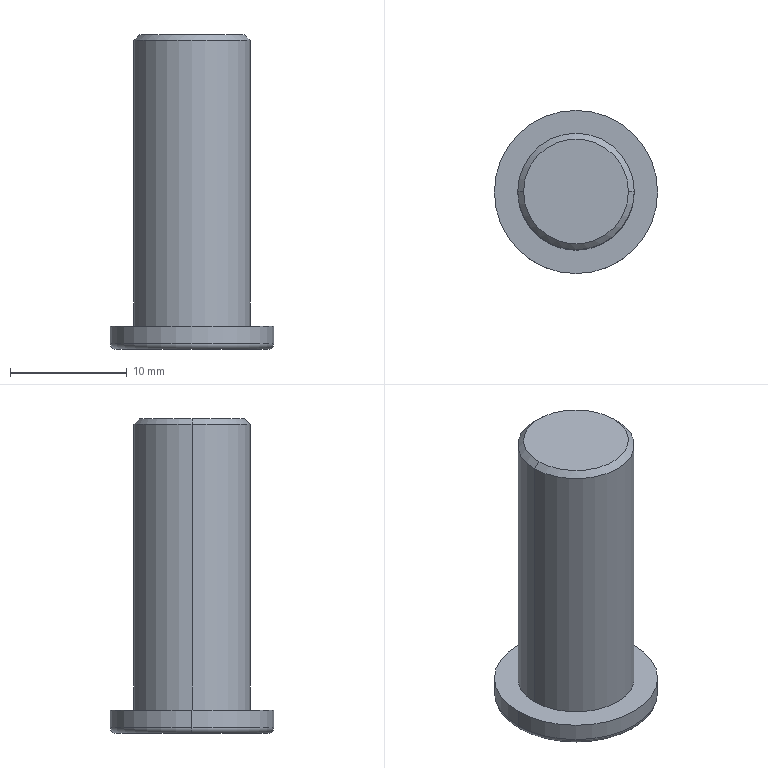Part | STEP file | BCC3 H11_4 | 1 solid | 11 faces | box 14 x 14 x 27 mm | volume 2265 mm3 | cylinder 4 | plane 3 | torus 2 | cone 2 | commonest cylinder face diameters 10 x2 14 x2
STEP:
#1=CARTESIAN_POINT('',(0.,0.,0.));
#2=DIRECTION('',(0.,0.,1.));
#3=DIRECTION('',(1.,0.,0.));
#4=AXIS2_PLACEMENT_3D('',#1,#2,#3);
#5=CARTESIAN_POINT('',(-6.5,0.,-2.));
#6=VERTEX_POINT('',#5);
#7=CARTESIAN_POINT('',(6.5,0.,-2.));
#8=VERTEX_POINT('',#7);
#9=CARTESIAN_POINT('',(0.,0.,-2.));
#10=DIRECTION('',(0.,0.,-1.));
#11=DIRECTION('',(1.,0.,0.));
#12=AXIS2_PLACEMENT_3D('',#9,#10,#11);
#13=CIRCLE('',#12,6.5);
#14=CARTESIAN_POINT('',(0.,0.,-1.5));
#15=DIRECTION('',(0.,0.,1.));
#16=DIRECTION('',(1.,0.,0.));
#17=AXIS2_PLACEMENT_3D('',#14,#15,#16);
#18=TOROIDAL_SURFACE('',#17,6.5,0.5);
#19=CARTESIAN_POINT('',(6.283,4.712));
#20=DIRECTION('',(-1.,0.));
#21=VECTOR('',#20,1.);
#22=LINE('',#19,#21);
#23=(GEOMETRIC_REPRESENTATION_CONTEXT(2)PARAMETRIC_REPRESENTATION_CONTEXT()REPRESENTATION_CONTEXT('',''));
#24=DEFINITIONAL_REPRESENTATION('',(#22),#23);
#25=PCURVE('',#18,#24);
#26=CARTESIAN_POINT('',(0.,0.,-2.));
#27=DIRECTION('',(0.,0.,1.));
#28=DIRECTION('',(1.,0.,0.));
#29=AXIS2_PLACEMENT_3D('',#26,#27,#28);
#30=PLANE('',#29);
#31=CARTESIAN_POINT('',(6.5,0.));
#32=CARTESIAN_POINT('',(6.5,-11.258));
#33=CARTESIAN_POINT('',(-3.25,-5.629));
#34=CARTESIAN_POINT('',(-13.,0.));
#35=CARTESIAN_POINT('',(-3.25,5.629));
#36=CARTESIAN_POINT('',(6.5,11.258));
#37=CARTESIAN_POINT('',(6.5,0.));
#38=(BOUNDED_CURVE()B_SPLINE_CURVE(2,(#31,#32,#33,#34,#35,#36,#37),.UNSPECIFIED.,.T.,.F.)B_SPLINE_CURVE_WITH_KNOTS((1,2,2,2,2,1),(-2.094,0.,2.094,4.189,6.283,8.378),.UNSPECIFIED.)CURVE()GEOMETRIC_REPRESENTATION_ITEM()RATIONAL_B_SPLINE_CURVE((1.,0.5,1.,0.5,1.,0.5,1.))REPRESENTATION_ITEM(''));
#39=(GEOMETRIC_REPRESENTATION_CONTEXT(2)PARAMETRIC_REPRESENTATION_CONTEXT()REPRESENTATION_CONTEXT('',''));
#40=DEFINITIONAL_REPRESENTATION('',(#38),#39);
#41=PCURVE('',#30,#40);
#42=SURFACE_CURVE('',#13,(#25,#41),.PCURVE_S1.);
#43=EDGE_CURVE('',#6,#8,#42,.T.);
#44=ORIENTED_EDGE('',*,*,#43,.F.);
#45=CARTESIAN_POINT('',(-7.,0.,-1.5));
#46=VERTEX_POINT('',#45);
#47=CARTESIAN_POINT('',(-6.5,0.,-1.5));
#48=DIRECTION('',(0.,1.,0.));
#49=DIRECTION('',(-1.,0.,0.));
#50=AXIS2_PLACEMENT_3D('',#47,#48,#49);
#51=CIRCLE('',#50,0.5);
#52=CARTESIAN_POINT('',(3.142,0.));
#53=DIRECTION('',(0.,1.));
#54=VECTOR('',#53,1.);
#55=LINE('',#52,#54);
#56=(GEOMETRIC_REPRESENTATION_CONTEXT(2)PARAMETRIC_REPRESENTATION_CONTEXT()REPRESENTATION_CONTEXT('',''));
#57=DEFINITIONAL_REPRESENTATION('',(#55),#56);
#58=PCURVE('',#18,#57);
#59=CARTESIAN_POINT('',(0.,0.,-1.5));
#60=DIRECTION('',(0.,0.,1.));
#61=DIRECTION('',(1.,0.,0.));
#62=AXIS2_PLACEMENT_3D('',#59,#60,#61);
#63=TOROIDAL_SURFACE('',#62,6.5,0.5);
#64=CARTESIAN_POINT('',(3.142,0.));
#65=DIRECTION('',(0.,1.));
#66=VECTOR('',#65,1.);
#67=LINE('',#64,#66);
#68=(GEOMETRIC_REPRESENTATION_CONTEXT(2)PARAMETRIC_REPRESENTATION_CONTEXT()REPRESENTATION_CONTEXT('',''));
#69=DEFINITIONAL_REPRESENTATION('',(#67),#68);
#70=PCURVE('',#63,#69);
#71=SURFACE_CURVE('',#51,(#58,#70),.PCURVE_S1.);
#72=EDGE_CURVE('',#6,#46,#71,.T.);
#73=ORIENTED_EDGE('',*,*,#72,.T.);
#74=CARTESIAN_POINT('',(7.,0.,-1.5));
#75=VERTEX_POINT('',#74);
#76=CARTESIAN_POINT('',(0.,0.,-1.5));
#77=DIRECTION('',(0.,0.,1.));
#78=DIRECTION('',(1.,0.,0.));
#79=AXIS2_PLACEMENT_3D('',#76,#77,#78);
#80=CIRCLE('',#79,7.);
#81=CARTESIAN_POINT('',(0.,6.283));
#82=DIRECTION('',(1.,0.));
#83=VECTOR('',#82,1.);
#84=LINE('',#81,#83);
#85=(GEOMETRIC_REPRESENTATION_CONTEXT(2)PARAMETRIC_REPRESENTATION_CONTEXT()REPRESENTATION_CONTEXT('',''));
#86=DEFINITIONAL_REPRESENTATION('',(#84),#85);
#87=PCURVE('',#18,#86);
#88=CARTESIAN_POINT('',(0.,0.,-2.));
#89=DIRECTION('',(0.,0.,1.));
#90=DIRECTION('',(1.,0.,0.));
#91=AXIS2_PLACEMENT_3D('',#88,#89,#90);
#92=CYLINDRICAL_SURFACE('',#91,7.);
#93=CARTESIAN_POINT('',(0.,0.5));
#94=DIRECTION('',(1.,0.));
#95=VECTOR('',#94,1.);
#96=LINE('',#93,#95);
#97=(GEOMETRIC_REPRESENTATION_CONTEXT(2)PARAMETRIC_REPRESENTATION_CONTEXT()REPRESENTATION_CONTEXT('',''));
#98=DEFINITIONAL_REPRESENTATION('',(#96),#97);
#99=PCURVE('',#92,#98);
#100=SURFACE_CURVE('',#80,(#87,#99),.PCURVE_S1.);
#101=EDGE_CURVE('',#75,#46,#100,.T.);
#102=ORIENTED_EDGE('',*,*,#101,.F.);
#103=CARTESIAN_POINT('',(6.5,0.,-1.5));
#104=DIRECTION('',(0.,-1.,0.));
#105=DIRECTION('',(0.,0.,-1.));
#106=AXIS2_PLACEMENT_3D('',#103,#104,#105);
#107=CIRCLE('',#106,0.5);
#108=CARTESIAN_POINT('',(0.,4.712));
#109=DIRECTION('',(0.,1.));
#110=VECTOR('',#109,1.);
#111=LINE('',#108,#110);
#112=(GEOMETRIC_REPRESENTATION_CONTEXT(2)PARAMETRIC_REPRESENTATION_CONTEXT()REPRESENTATION_CONTEXT('',''));
#113=DEFINITIONAL_REPRESENTATION('',(#111),#112);
#114=PCURVE('',#18,#113);
#115=CARTESIAN_POINT('',(6.283,4.712));
#116=DIRECTION('',(0.,1.));
#117=VECTOR('',#116,1.);
#118=LINE('',#115,#117);
#119=(GEOMETRIC_REPRESENTATION_CONTEXT(2)PARAMETRIC_REPRESENTATION_CONTEXT()REPRESENTATION_CONTEXT('',''));
#120=DEFINITIONAL_REPRESENTATION('',(#118),#119);
#121=PCURVE('',#63,#120);
#122=SURFACE_CURVE('',#107,(#114,#121),.PCURVE_S1.);
#123=EDGE_CURVE('',#8,#75,#122,.T.);
#124=ORIENTED_EDGE('',*,*,#123,.F.);
#125=EDGE_LOOP('',(#44,#73,#102,#124));
#126=FACE_BOUND('',#125,.T.);
#127=ADVANCED_FACE('',(#126),#18,.T.);
#128=CARTESIAN_POINT('',(4.5,0.,25.));
#129=VERTEX_POINT('',#128);
#130=CARTESIAN_POINT('',(-4.5,0.,25.));
#131=VERTEX_POINT('',#130);
#132=CARTESIAN_POINT('',(0.,0.,25.));
#133=DIRECTION('',(0.,0.,1.));
#134=DIRECTION('',(1.,0.,0.));
#135=AXIS2_PLACEMENT_3D('',#132,#133,#134);
#136=CIRCLE('',#135,4.5);
#137=CARTESIAN_POINT('',(0.,0.,25.));
#138=DIRECTION('',(0.,0.,-1.));
#139=DIRECTION('',(-1.,0.,0.));
#140=AXIS2_PLACEMENT_3D('',#137,#138,#139);
#141=CONICAL_SURFACE('',#140,4.5,0.7854);
#142=CARTESIAN_POINT('',(3.142,0.));
#143=DIRECTION('',(-1.,0.));
#144=VECTOR('',#143,1.);
#145=LINE('',#142,#144);
#146=(GEOMETRIC_REPRESENTATION_CONTEXT(2)PARAMETRIC_REPRESENTATION_CONTEXT()REPRESENTATION_CONTEXT('',''));
#147=DEFINITIONAL_REPRESENTATION('',(#145),#146);
#148=PCURVE('',#141,#147);
#149=CARTESIAN_POINT('',(0.,0.,25.));
#150=DIRECTION('',(0.,0.,1.));
#151=DIRECTION('',(1.,0.,0.));
#152=AXIS2_PLACEMENT_3D('',#149,#150,#151);
#153=PLANE('',#152);
#154=CARTESIAN_POINT('',(0.,0.));
#155=DIRECTION('',(1.,0.));
#156=AXIS2_PLACEMENT_2D('',#154,#155);
#157=CIRCLE('',#156,4.5);
#158=(GEOMETRIC_REPRESENTATION_CONTEXT(2)PARAMETRIC_REPRESENTATION_CONTEXT()REPRESENTATION_CONTEXT('',''));
#159=DEFINITIONAL_REPRESENTATION('',(#157),#158);
#160=PCURVE('',#153,#159);
#161=SURFACE_CURVE('',#136,(#148,#160),.PCURVE_S1.);
#162=EDGE_CURVE('',#129,#131,#161,.T.);
#163=ORIENTED_EDGE('',*,*,#162,.F.);
#164=CARTESIAN_POINT('',(5.,0.,24.5));
#165=VERTEX_POINT('',#164);
#166=CARTESIAN_POINT('',(4.5,0.,25.));
#167=DIRECTION('',(0.7071,0.,-0.7071));
#168=VECTOR('',#167,1.);
#169=LINE('',#166,#168);
#170=CARTESIAN_POINT('',(3.142,0.));
#171=DIRECTION('',(0.,1.));
#172=VECTOR('',#171,1.);
#173=LINE('',#170,#172);
#174=(GEOMETRIC_REPRESENTATION_CONTEXT(2)PARAMETRIC_REPRESENTATION_CONTEXT()REPRESENTATION_CONTEXT('',''));
#175=DEFINITIONAL_REPRESENTATION('',(#173),#174);
#176=PCURVE('',#141,#175);
#177=CARTESIAN_POINT('',(0.,0.,25.));
#178=DIRECTION('',(0.,0.,-1.));
#179=DIRECTION('',(-1.,0.,0.));
#180=AXIS2_PLACEMENT_3D('',#177,#178,#179);
#181=CONICAL_SURFACE('',#180,4.5,0.7854);
#182=CARTESIAN_POINT('',(3.142,0.));
#183=DIRECTION('',(0.,1.));
#184=VECTOR('',#183,1.);
#185=LINE('',#182,#184);
#186=(GEOMETRIC_REPRESENTATION_CONTEXT(2)PARAMETRIC_REPRESENTATION_CONTEXT()REPRESENTATION_CONTEXT('',''));
#187=DEFINITIONAL_REPRESENTATION('',(#185),#186);
#188=PCURVE('',#181,#187);
#189=SURFACE_CURVE('',#169,(#176,#188),.PCURVE_S1.);
#190=EDGE_CURVE('',#129,#165,#189,.T.);
#191=ORIENTED_EDGE('',*,*,#190,.T.);
#192=CARTESIAN_POINT('',(-5.,0.,24.5));
#193=VERTEX_POINT('',#192);
#194=CARTESIAN_POINT('',(0.,0.,24.5));
#195=DIRECTION('',(0.,0.,-1.));
#196=DIRECTION('',(1.,0.,0.));
#197=AXIS2_PLACEMENT_3D('',#194,#195,#196);
#198=CIRCLE('',#197,5.);
#199=CARTESIAN_POINT('',(-3.142,0.5));
#200=DIRECTION('',(1.,0.));
#201=VECTOR('',#200,1.);
#202=LINE('',#199,#201);
#203=(GEOMETRIC_REPRESENTATION_CONTEXT(2)PARAMETRIC_REPRESENTATION_CONTEXT()REPRESENTATION_CONTEXT('',''));
#204=DEFINITIONAL_REPRESENTATION('',(#202),#203);
#205=PCURVE('',#141,#204);
#206=CARTESIAN_POINT('',(0.,0.,25.));
#207=DIRECTION('',(0.,0.,-1.));
#208=DIRECTION('',(-1.,0.,0.));
#209=AXIS2_PLACEMENT_3D('',#206,#207,#208);
#210=CYLINDRICAL_SURFACE('',#209,5.);
#211=CARTESIAN_POINT('',(-3.142,0.5));
#212=DIRECTION('',(1.,0.));
#213=VECTOR('',#212,1.);
#214=LINE('',#211,#213);
#215=(GEOMETRIC_REPRESENTATION_CONTEXT(2)PARAMETRIC_REPRESENTATION_CONTEXT()REPRESENTATION_CONTEXT('',''));
#216=DEFINITIONAL_REPRESENTATION('',(#214),#215);
#217=PCURVE('',#210,#216);
#218=SURFACE_CURVE('',#198,(#205,#217),.PCURVE_S1.);
#219=EDGE_CURVE('',#193,#165,#218,.T.);
#220=ORIENTED_EDGE('',*,*,#219,.F.);
#221=CARTESIAN_POINT('',(-4.5,0.,25.));
#222=DIRECTION('',(-0.7071,0.,-0.7071));
#223=VECTOR('',#222,1.);
#224=LINE('',#221,#223);
#225=CARTESIAN_POINT('',(0.,0.));
#226=DIRECTION('',(0.,1.));
#227=VECTOR('',#226,1.);
#228=LINE('',#225,#227);
#229=(GEOMETRIC_REPRESENTATION_CONTEXT(2)PARAMETRIC_REPRESENTATION_CONTEXT()REPRESENTATION_CONTEXT('',''));
#230=DEFINITIONAL_REPRESENTATION('',(#228),#229);
#231=PCURVE('',#141,#230);
#232=CARTESIAN_POINT('',(6.283,0.));
#233=DIRECTION('',(0.,1.));
#234=VECTOR('',#233,1.);
#235=LINE('',#232,#234);
#236=(GEOMETRIC_REPRESENTATION_CONTEXT(2)PARAMETRIC_REPRESENTATION_CONTEXT()REPRESENTATION_CONTEXT('',''));
#237=DEFINITIONAL_REPRESENTATION('',(#235),#236);
#238=PCURVE('',#181,#237);
#239=SURFACE_CURVE('',#224,(#231,#238),.PCURVE_S1.);
#240=EDGE_CURVE('',#131,#193,#239,.T.);
#241=ORIENTED_EDGE('',*,*,#240,.F.);
#242=EDGE_LOOP('',(#163,#191,#220,#241));
#243=FACE_BOUND('',#242,.T.);
#244=ADVANCED_FACE('',(#243),#141,.T.);
#245=ORIENTED_EDGE('',*,*,#219,.T.);
#246=CARTESIAN_POINT('',(5.,0.,0.));
#247=VERTEX_POINT('',#246);
#248=CARTESIAN_POINT('',(5.,0.,25.));
#249=DIRECTION('',(0.,0.,-1.));
#250=VECTOR('',#249,1.);
#251=LINE('',#248,#250);
#252=CARTESIAN_POINT('',(3.142,0.));
#253=DIRECTION('',(0.,1.));
#254=VECTOR('',#253,1.);
#255=LINE('',#252,#254);
#256=(GEOMETRIC_REPRESENTATION_CONTEXT(2)PARAMETRIC_REPRESENTATION_CONTEXT()REPRESENTATION_CONTEXT('',''));
#257=DEFINITIONAL_REPRESENTATION('',(#255),#256);
#258=PCURVE('',#210,#257);
#259=CARTESIAN_POINT('',(0.,0.,25.));
#260=DIRECTION('',(0.,0.,-1.));
#261=DIRECTION('',(-1.,0.,0.));
#262=AXIS2_PLACEMENT_3D('',#259,#260,#261);
#263=CYLINDRICAL_SURFACE('',#262,5.);
#264=CARTESIAN_POINT('',(3.142,0.));
#265=DIRECTION('',(0.,1.));
#266=VECTOR('',#265,1.);
#267=LINE('',#264,#266);
#268=(GEOMETRIC_REPRESENTATION_CONTEXT(2)PARAMETRIC_REPRESENTATION_CONTEXT()REPRESENTATION_CONTEXT('',''));
#269=DEFINITIONAL_REPRESENTATION('',(#267),#268);
#270=PCURVE('',#263,#269);
#271=SURFACE_CURVE('',#251,(#258,#270),.PCURVE_S1.);
#272=EDGE_CURVE('',#165,#247,#271,.T.);
#273=ORIENTED_EDGE('',*,*,#272,.T.);
#274=CARTESIAN_POINT('',(-5.,0.,0.));
#275=VERTEX_POINT('',#274);
#276=CARTESIAN_POINT('',(0.,0.,0.));
#277=DIRECTION('',(0.,0.,1.));
#278=DIRECTION('',(1.,0.,0.));
#279=AXIS2_PLACEMENT_3D('',#276,#277,#278);
#280=CIRCLE('',#279,5.);
#281=CARTESIAN_POINT('',(3.142,25.));
#282=DIRECTION('',(-1.,0.));
#283=VECTOR('',#282,1.);
#284=LINE('',#281,#283);
#285=(GEOMETRIC_REPRESENTATION_CONTEXT(2)PARAMETRIC_REPRESENTATION_CONTEXT()REPRESENTATION_CONTEXT('',''));
#286=DEFINITIONAL_REPRESENTATION('',(#284),#285);
#287=PCURVE('',#210,#286);
#288=CARTESIAN_POINT('',(0.,0.,0.));
#289=DIRECTION('',(0.,0.,1.));
#290=DIRECTION('',(1.,0.,0.));
#291=AXIS2_PLACEMENT_3D('',#288,#289,#290);
#292=PLANE('',#291);
#293=CARTESIAN_POINT('',(0.,0.));
#294=DIRECTION('',(1.,0.));
#295=AXIS2_PLACEMENT_2D('',#293,#294);
#296=CIRCLE('',#295,5.);
#297=(GEOMETRIC_REPRESENTATION_CONTEXT(2)PARAMETRIC_REPRESENTATION_CONTEXT()REPRESENTATION_CONTEXT('',''));
#298=DEFINITIONAL_REPRESENTATION('',(#296),#297);
#299=PCURVE('',#292,#298);
#300=SURFACE_CURVE('',#280,(#287,#299),.PCURVE_S1.);
#301=EDGE_CURVE('',#247,#275,#300,.T.);
#302=ORIENTED_EDGE('',*,*,#301,.T.);
#303=CARTESIAN_POINT('',(-5.,0.,25.));
#304=DIRECTION('',(0.,0.,-1.));
#305=VECTOR('',#304,1.);
#306=LINE('',#303,#305);
#307=CARTESIAN_POINT('',(0.,0.));
#308=DIRECTION('',(0.,1.));
#309=VECTOR('',#308,1.);
#310=LINE('',#307,#309);
#311=(GEOMETRIC_REPRESENTATION_CONTEXT(2)PARAMETRIC_REPRESENTATION_CONTEXT()REPRESENTATION_CONTEXT('',''));
#312=DEFINITIONAL_REPRESENTATION('',(#310),#311);
#313=PCURVE('',#210,#312);
#314=CARTESIAN_POINT('',(6.283,0.));
#315=DIRECTION('',(0.,1.));
#316=VECTOR('',#315,1.);
#317=LINE('',#314,#316);
#318=(GEOMETRIC_REPRESENTATION_CONTEXT(2)PARAMETRIC_REPRESENTATION_CONTEXT()REPRESENTATION_CONTEXT('',''));
#319=DEFINITIONAL_REPRESENTATION('',(#317),#318);
#320=PCURVE('',#263,#319);
#321=SURFACE_CURVE('',#306,(#313,#320),.PCURVE_S1.);
#322=EDGE_CURVE('',#193,#275,#321,.T.);
#323=ORIENTED_EDGE('',*,*,#322,.F.);
#324=EDGE_LOOP('',(#245,#273,#302,#323));
#325=FACE_BOUND('',#324,.T.);
#326=ADVANCED_FACE('',(#325),#210,.T.);
#327=ORIENTED_EDGE('',*,*,#101,.T.);
#328=CARTESIAN_POINT('',(-7.,0.,0.));
#329=VERTEX_POINT('',#328);
#330=CARTESIAN_POINT('',(-7.,0.,-2.));
#331=DIRECTION('',(0.,0.,1.));
#332=VECTOR('',#331,1.);
#333=LINE('',#330,#332);
#334=CARTESIAN_POINT('',(3.142,0.));
#335=DIRECTION('',(0.,1.));
#336=VECTOR('',#335,1.);
#337=LINE('',#334,#336);
#338=(GEOMETRIC_REPRESENTATION_CONTEXT(2)PARAMETRIC_REPRESENTATION_CONTEXT()REPRESENTATION_CONTEXT('',''));
#339=DEFINITIONAL_REPRESENTATION('',(#337),#338);
#340=PCURVE('',#92,#339);
#341=CARTESIAN_POINT('',(0.,0.,-2.));
#342=DIRECTION('',(0.,0.,1.));
#343=DIRECTION('',(1.,0.,0.));
#344=AXIS2_PLACEMENT_3D('',#341,#342,#343);
#345=CYLINDRICAL_SURFACE('',#344,7.);
#346=CARTESIAN_POINT('',(3.142,0.));
#347=DIRECTION('',(0.,1.));
#348=VECTOR('',#347,1.);
#349=LINE('',#346,#348);
#350=(GEOMETRIC_REPRESENTATION_CONTEXT(2)PARAMETRIC_REPRESENTATION_CONTEXT()REPRESENTATION_CONTEXT('',''));
#351=DEFINITIONAL_REPRESENTATION('',(#349),#350);
#352=PCURVE('',#345,#351);
#353=SURFACE_CURVE('',#333,(#340,#352),.PCURVE_S1.);
#354=EDGE_CURVE('',#46,#329,#353,.T.);
#355=ORIENTED_EDGE('',*,*,#354,.T.);
#356=CARTESIAN_POINT('',(7.,0.,0.));
#357=VERTEX_POINT('',#356);
#358=CARTESIAN_POINT('',(0.,0.,0.));
#359=DIRECTION('',(0.,0.,1.));
#360=DIRECTION('',(1.,0.,0.));
#361=AXIS2_PLACEMENT_3D('',#358,#359,#360);
#362=CIRCLE('',#361,7.);
#363=CARTESIAN_POINT('',(0.,2.));
#364=DIRECTION('',(1.,0.));
#365=VECTOR('',#364,1.);
#366=LINE('',#363,#365);
#367=(GEOMETRIC_REPRESENTATION_CONTEXT(2)PARAMETRIC_REPRESENTATION_CONTEXT()REPRESENTATION_CONTEXT('',''));
#368=DEFINITIONAL_REPRESENTATION('',(#366),#367);
#369=PCURVE('',#92,#368);
#370=CARTESIAN_POINT('',(0.,0.));
#371=DIRECTION('',(1.,0.));
#372=AXIS2_PLACEMENT_2D('',#370,#371);
#373=CIRCLE('',#372,7.);
#374=(GEOMETRIC_REPRESENTATION_CONTEXT(2)PARAMETRIC_REPRESENTATION_CONTEXT()REPRESENTATION_CONTEXT('',''));
#375=DEFINITIONAL_REPRESENTATION('',(#373),#374);
#376=PCURVE('',#292,#375);
#377=SURFACE_CURVE('',#362,(#369,#376),.PCURVE_S1.);
#378=EDGE_CURVE('',#357,#329,#377,.T.);
#379=ORIENTED_EDGE('',*,*,#378,.F.);
#380=CARTESIAN_POINT('',(7.,0.,-2.));
#381=DIRECTION('',(0.,0.,1.));
#382=VECTOR('',#381,1.);
#383=LINE('',#380,#382);
#384=CARTESIAN_POINT('',(0.,0.));
#385=DIRECTION('',(0.,1.));
#386=VECTOR('',#385,1.);
#387=LINE('',#384,#386);
#388=(GEOMETRIC_REPRESENTATION_CONTEXT(2)PARAMETRIC_REPRESENTATION_CONTEXT()REPRESENTATION_CONTEXT('',''));
#389=DEFINITIONAL_REPRESENTATION('',(#387),#388);
#390=PCURVE('',#92,#389);
#391=CARTESIAN_POINT('',(6.283,0.));
#392=DIRECTION('',(0.,1.));
#393=VECTOR('',#392,1.);
#394=LINE('',#391,#393);
#395=(GEOMETRIC_REPRESENTATION_CONTEXT(2)PARAMETRIC_REPRESENTATION_CONTEXT()REPRESENTATION_CONTEXT('',''));
#396=DEFINITIONAL_REPRESENTATION('',(#394),#395);
#397=PCURVE('',#345,#396);
#398=SURFACE_CURVE('',#383,(#390,#397),.PCURVE_S1.);
#399=EDGE_CURVE('',#75,#357,#398,.T.);
#400=ORIENTED_EDGE('',*,*,#399,.F.);
#401=EDGE_LOOP('',(#327,#355,#379,#400));
#402=FACE_BOUND('',#401,.T.);
#403=ADVANCED_FACE('',(#402),#92,.T.);
#404=ORIENTED_EDGE('',*,*,#378,.T.);
#405=CARTESIAN_POINT('',(0.,0.,0.));
#406=DIRECTION('',(0.,0.,1.));
#407=DIRECTION('',(1.,0.,0.));
#408=AXIS2_PLACEMENT_3D('',#405,#406,#407);
#409=CIRCLE('',#408,7.);
#410=CARTESIAN_POINT('',(0.,0.));
#411=DIRECTION('',(1.,0.));
#412=AXIS2_PLACEMENT_2D('',#410,#411);
#413=CIRCLE('',#412,7.);
#414=(GEOMETRIC_REPRESENTATION_CONTEXT(2)PARAMETRIC_REPRESENTATION_CONTEXT()REPRESENTATION_CONTEXT('',''));
#415=DEFINITIONAL_REPRESENTATION('',(#413),#414);
#416=PCURVE('',#292,#415);
#417=CARTESIAN_POINT('',(0.,2.));
#418=DIRECTION('',(1.,0.));
#419=VECTOR('',#418,1.);
#420=LINE('',#417,#419);
#421=(GEOMETRIC_REPRESENTATION_CONTEXT(2)PARAMETRIC_REPRESENTATION_CONTEXT()REPRESENTATION_CONTEXT('',''));
#422=DEFINITIONAL_REPRESENTATION('',(#420),#421);
#423=PCURVE('',#345,#422);
#424=SURFACE_CURVE('',#409,(#416,#423),.PCURVE_S1.);
#425=EDGE_CURVE('',#329,#357,#424,.T.);
#426=ORIENTED_EDGE('',*,*,#425,.T.);
#427=EDGE_LOOP('',(#404,#426));
#428=FACE_BOUND('',#427,.T.);
#429=CARTESIAN_POINT('',(0.,0.,0.));
#430=DIRECTION('',(0.,0.,1.));
#431=DIRECTION('',(1.,0.,0.));
#432=AXIS2_PLACEMENT_3D('',#429,#430,#431);
#433=CIRCLE('',#432,5.);
#434=CARTESIAN_POINT('',(0.,0.));
#435=DIRECTION('',(1.,0.));
#436=AXIS2_PLACEMENT_2D('',#434,#435);
#437=CIRCLE('',#436,5.);
#438=(GEOMETRIC_REPRESENTATION_CONTEXT(2)PARAMETRIC_REPRESENTATION_CONTEXT()REPRESENTATION_CONTEXT('',''));
#439=DEFINITIONAL_REPRESENTATION('',(#437),#438);
#440=PCURVE('',#292,#439);
#441=CARTESIAN_POINT('',(9.425,25.));
#442=DIRECTION('',(-1.,0.));
#443=VECTOR('',#442,1.);
#444=LINE('',#441,#443);
#445=(GEOMETRIC_REPRESENTATION_CONTEXT(2)PARAMETRIC_REPRESENTATION_CONTEXT()REPRESENTATION_CONTEXT('',''));
#446=DEFINITIONAL_REPRESENTATION('',(#444),#445);
#447=PCURVE('',#263,#446);
#448=SURFACE_CURVE('',#433,(#440,#447),.PCURVE_S1.);
#449=EDGE_CURVE('',#275,#247,#448,.T.);
#450=ORIENTED_EDGE('',*,*,#449,.F.);
#451=ORIENTED_EDGE('',*,*,#301,.F.);
#452=EDGE_LOOP('',(#450,#451));
#453=FACE_BOUND('',#452,.T.);
#454=ADVANCED_FACE('',(#428,#453),#292,.T.);
#455=ORIENTED_EDGE('',*,*,#354,.F.);
#456=CARTESIAN_POINT('',(0.,0.,-1.5));
#457=DIRECTION('',(0.,0.,1.));
#458=DIRECTION('',(1.,0.,0.));
#459=AXIS2_PLACEMENT_3D('',#456,#457,#458);
#460=CIRCLE('',#459,7.);
#461=CARTESIAN_POINT('',(0.,0.5));
#462=DIRECTION('',(1.,0.));
#463=VECTOR('',#462,1.);
#464=LINE('',#461,#463);
#465=(GEOMETRIC_REPRESENTATION_CONTEXT(2)PARAMETRIC_REPRESENTATION_CONTEXT()REPRESENTATION_CONTEXT('',''));
#466=DEFINITIONAL_REPRESENTATION('',(#464),#465);
#467=PCURVE('',#345,#466);
#468=CARTESIAN_POINT('',(0.,6.283));
#469=DIRECTION('',(1.,0.));
#470=VECTOR('',#469,1.);
#471=LINE('',#468,#470);
#472=(GEOMETRIC_REPRESENTATION_CONTEXT(2)PARAMETRIC_REPRESENTATION_CONTEXT()REPRESENTATION_CONTEXT('',''));
#473=DEFINITIONAL_REPRESENTATION('',(#471),#472);
#474=PCURVE('',#63,#473);
#475=SURFACE_CURVE('',#460,(#467,#474),.PCURVE_S1.);
#476=EDGE_CURVE('',#46,#75,#475,.T.);
#477=ORIENTED_EDGE('',*,*,#476,.T.);
#478=ORIENTED_EDGE('',*,*,#399,.T.);
#479=ORIENTED_EDGE('',*,*,#425,.F.);
#480=EDGE_LOOP('',(#455,#477,#478,#479));
#481=FACE_BOUND('',#480,.T.);
#482=ADVANCED_FACE('',(#481),#345,.T.);
#483=CARTESIAN_POINT('',(0.,0.,-2.));
#484=DIRECTION('',(0.,0.,-1.));
#485=DIRECTION('',(1.,0.,0.));
#486=AXIS2_PLACEMENT_3D('',#483,#484,#485);
#487=CIRCLE('',#486,6.5);
#488=CARTESIAN_POINT('',(6.5,0.));
#489=CARTESIAN_POINT('',(6.5,-11.258));
#490=CARTESIAN_POINT('',(-3.25,-5.629));
#491=CARTESIAN_POINT('',(-13.,0.));
#492=CARTESIAN_POINT('',(-3.25,5.629));
#493=CARTESIAN_POINT('',(6.5,11.258));
#494=CARTESIAN_POINT('',(6.5,0.));
#495=(BOUNDED_CURVE()B_SPLINE_CURVE(2,(#488,#489,#490,#491,#492,#493,#494),.UNSPECIFIED.,.T.,.F.)B_SPLINE_CURVE_WITH_KNOTS((1,2,2,2,2,1),(-2.094,0.,2.094,4.189,6.283,8.378),.UNSPECIFIED.)CURVE()GEOMETRIC_REPRESENTATION_ITEM()RATIONAL_B_SPLINE_CURVE((1.,0.5,1.,0.5,1.,0.5,1.))REPRESENTATION_ITEM(''));
#496=(GEOMETRIC_REPRESENTATION_CONTEXT(2)PARAMETRIC_REPRESENTATION_CONTEXT()REPRESENTATION_CONTEXT('',''));
#497=DEFINITIONAL_REPRESENTATION('',(#495),#496);
#498=PCURVE('',#30,#497);
#499=CARTESIAN_POINT('',(6.283,4.712));
#500=DIRECTION('',(-1.,0.));
#501=VECTOR('',#500,1.);
#502=LINE('',#499,#501);
#503=(GEOMETRIC_REPRESENTATION_CONTEXT(2)PARAMETRIC_REPRESENTATION_CONTEXT()REPRESENTATION_CONTEXT('',''));
#504=DEFINITIONAL_REPRESENTATION('',(#502),#503);
#505=PCURVE('',#63,#504);
#506=SURFACE_CURVE('',#487,(#498,#505),.PCURVE_S1.);
#507=EDGE_CURVE('',#8,#6,#506,.T.);
#508=ORIENTED_EDGE('',*,*,#507,.T.);
#509=ORIENTED_EDGE('',*,*,#43,.T.);
#510=EDGE_LOOP('',(#508,#509));
#511=FACE_BOUND('',#510,.T.);
#512=ADVANCED_FACE('',(#511),#30,.F.);
#513=ORIENTED_EDGE('',*,*,#272,.F.);
#514=CARTESIAN_POINT('',(0.,0.,24.5));
#515=DIRECTION('',(0.,0.,-1.));
#516=DIRECTION('',(1.,0.,0.));
#517=AXIS2_PLACEMENT_3D('',#514,#515,#516);
#518=CIRCLE('',#517,5.);
#519=CARTESIAN_POINT('',(3.142,0.5));
#520=DIRECTION('',(1.,0.));
#521=VECTOR('',#520,1.);
#522=LINE('',#519,#521);
#523=(GEOMETRIC_REPRESENTATION_CONTEXT(2)PARAMETRIC_REPRESENTATION_CONTEXT()REPRESENTATION_CONTEXT('',''));
#524=DEFINITIONAL_REPRESENTATION('',(#522),#523);
#525=PCURVE('',#263,#524);
#526=CARTESIAN_POINT('',(3.142,0.5));
#527=DIRECTION('',(1.,0.));
#528=VECTOR('',#527,1.);
#529=LINE('',#526,#528);
#530=(GEOMETRIC_REPRESENTATION_CONTEXT(2)PARAMETRIC_REPRESENTATION_CONTEXT()REPRESENTATION_CONTEXT('',''));
#531=DEFINITIONAL_REPRESENTATION('',(#529),#530);
#532=PCURVE('',#181,#531);
#533=SURFACE_CURVE('',#518,(#525,#532),.PCURVE_S1.);
#534=EDGE_CURVE('',#165,#193,#533,.T.);
#535=ORIENTED_EDGE('',*,*,#534,.T.);
#536=ORIENTED_EDGE('',*,*,#322,.T.);
#537=ORIENTED_EDGE('',*,*,#449,.T.);
#538=EDGE_LOOP('',(#513,#535,#536,#537));
#539=FACE_BOUND('',#538,.T.);
#540=ADVANCED_FACE('',(#539),#263,.T.);
#541=CARTESIAN_POINT('',(0.,0.,25.));
#542=DIRECTION('',(0.,0.,1.));
#543=DIRECTION('',(1.,0.,0.));
#544=AXIS2_PLACEMENT_3D('',#541,#542,#543);
#545=CIRCLE('',#544,4.5);
#546=CARTESIAN_POINT('',(0.,0.));
#547=DIRECTION('',(1.,0.));
#548=AXIS2_PLACEMENT_2D('',#546,#547);
#549=CIRCLE('',#548,4.5);
#550=(GEOMETRIC_REPRESENTATION_CONTEXT(2)PARAMETRIC_REPRESENTATION_CONTEXT()REPRESENTATION_CONTEXT('',''));
#551=DEFINITIONAL_REPRESENTATION('',(#549),#550);
#552=PCURVE('',#153,#551);
#553=CARTESIAN_POINT('',(9.425,0.));
#554=DIRECTION('',(-1.,0.));
#555=VECTOR('',#554,1.);
#556=LINE('',#553,#555);
#557=(GEOMETRIC_REPRESENTATION_CONTEXT(2)PARAMETRIC_REPRESENTATION_CONTEXT()REPRESENTATION_CONTEXT('',''));
#558=DEFINITIONAL_REPRESENTATION('',(#556),#557);
#559=PCURVE('',#181,#558);
#560=SURFACE_CURVE('',#545,(#552,#559),.PCURVE_S1.);
#561=EDGE_CURVE('',#131,#129,#560,.T.);
#562=ORIENTED_EDGE('',*,*,#561,.T.);
#563=ORIENTED_EDGE('',*,*,#162,.T.);
#564=EDGE_LOOP('',(#562,#563));
#565=FACE_BOUND('',#564,.T.);
#566=ADVANCED_FACE('',(#565),#153,.T.);
#567=ORIENTED_EDGE('',*,*,#190,.F.);
#568=ORIENTED_EDGE('',*,*,#561,.F.);
#569=ORIENTED_EDGE('',*,*,#240,.T.);
#570=ORIENTED_EDGE('',*,*,#534,.F.);
#571=EDGE_LOOP('',(#567,#568,#569,#570));
#572=FACE_BOUND('',#571,.T.);
#573=ADVANCED_FACE('',(#572),#181,.T.);
#574=ORIENTED_EDGE('',*,*,#72,.F.);
#575=ORIENTED_EDGE('',*,*,#507,.F.);
#576=ORIENTED_EDGE('',*,*,#123,.T.);
#577=ORIENTED_EDGE('',*,*,#476,.F.);
#578=EDGE_LOOP('',(#574,#575,#576,#577));
#579=FACE_BOUND('',#578,.T.);
#580=ADVANCED_FACE('',(#579),#63,.T.);
#581=CLOSED_SHELL('',(#127,#244,#326,#403,#454,#482,#512,#540,#566,#573,#580));
#582=MANIFOLD_SOLID_BREP('',#581);
#583=(LENGTH_UNIT()NAMED_UNIT(*)SI_UNIT(.MILLI.,.METRE.));
#584=UNCERTAINTY_MEASURE_WITH_UNIT(LENGTH_MEASURE(0.0000001),#583,'','');
#585=(NAMED_UNIT(*)PLANE_ANGLE_UNIT()SI_UNIT($,.RADIAN.));
#586=(NAMED_UNIT(*)SI_UNIT($,.STERADIAN.)SOLID_ANGLE_UNIT());
#587=(GEOMETRIC_REPRESENTATION_CONTEXT(3)GLOBAL_UNCERTAINTY_ASSIGNED_CONTEXT((#584))GLOBAL_UNIT_ASSIGNED_CONTEXT((#583,#585,#586))REPRESENTATION_CONTEXT('',''));
#588=ADVANCED_BREP_SHAPE_REPRESENTATION('',(#4,#582),#587);